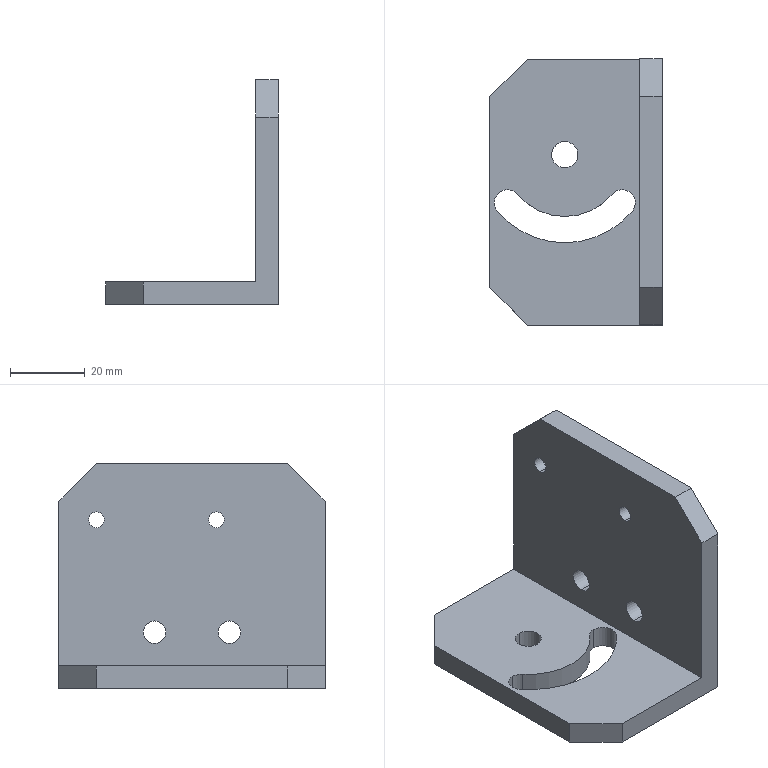Part | SolidWorks | features HoleWzd 3, ICE 2, Chamfer 1, Extrusion 1 | 1 solid | 28 faces | box 46 x 71 x 60 mm | volume 38967 mm3 | cylinder 16 | plane 12 | commonest cylinder face diameters 7 x6 4.2 x4 6 x4 33 x1 47 x1
STEP:
#1=CARTESIAN_POINT('',(-4.679,0.6442,-24.));
#2=VERTEX_POINT('',#1);
#3=CARTESIAN_POINT('',(-1.998,-5.106,-24.));
#4=VERTEX_POINT('',#3);
#5=CARTESIAN_POINT('',(-4.679,-2.856,-24.));
#6=DIRECTION('',(0.,0.,-1.));
#7=DIRECTION('',(0.,1.,0.));
#8=AXIS2_PLACEMENT_3D('',#5,#6,#7);
#9=CIRCLE('',#8,3.5);
#10=EDGE_CURVE('',#2,#4,#9,.T.);
#11=ORIENTED_EDGE('',*,*,#10,.F.);
#12=CARTESIAN_POINT('',(-4.679,0.6442,-30.));
#13=VERTEX_POINT('',#12);
#14=CARTESIAN_POINT('',(-4.679,0.6442,30.));
#15=DIRECTION('',(0.,0.,-1.));
#16=VECTOR('',#15,1000.);
#17=LINE('',#14,#16);
#18=EDGE_CURVE('',#2,#13,#17,.T.);
#19=ORIENTED_EDGE('',*,*,#18,.T.);
#20=CARTESIAN_POINT('',(-1.998,-5.106,-30.));
#21=VERTEX_POINT('',#20);
#22=CARTESIAN_POINT('',(-4.679,-2.856,-30.));
#23=DIRECTION('',(0.,0.,-1.));
#24=DIRECTION('',(0.,1.,0.));
#25=AXIS2_PLACEMENT_3D('',#22,#23,#24);
#26=CIRCLE('',#25,3.5);
#27=EDGE_CURVE('',#13,#21,#26,.T.);
#28=ORIENTED_EDGE('',*,*,#27,.T.);
#29=CARTESIAN_POINT('',(-1.998,-5.106,30.));
#30=DIRECTION('',(0.,0.,-1.));
#31=VECTOR('',#30,1000.);
#32=LINE('',#29,#31);
#33=EDGE_CURVE('',#4,#21,#32,.T.);
#34=ORIENTED_EDGE('',*,*,#33,.F.);
#35=EDGE_LOOP('',(#11,#19,#28,#34));
#36=FACE_OUTER_BOUND('',#35,.T.);
#37=CARTESIAN_POINT('',(-4.679,-2.856,30.));
#38=DIRECTION('',(0.,0.,-1.));
#39=DIRECTION('',(0.,1.,0.));
#40=AXIS2_PLACEMENT_3D('',#37,#38,#39);
#41=CYLINDRICAL_SURFACE('',#40,3.5);
#42=ADVANCED_FACE('',(#36),#41,.F.);
#43=CARTESIAN_POINT('',(-35.321,0.6442,-24.));
#44=VERTEX_POINT('',#43);
#45=CARTESIAN_POINT('',(-32.64,-0.606,-24.));
#46=VERTEX_POINT('',#45);
#47=CARTESIAN_POINT('',(-35.321,-2.856,-24.));
#48=DIRECTION('',(0.,0.,-1.));
#49=DIRECTION('',(0.,1.,0.));
#50=AXIS2_PLACEMENT_3D('',#47,#48,#49);
#51=CIRCLE('',#50,3.5);
#52=EDGE_CURVE('',#44,#46,#51,.T.);
#53=ORIENTED_EDGE('',*,*,#52,.F.);
#54=CARTESIAN_POINT('',(-35.321,0.6442,-30.));
#55=VERTEX_POINT('',#54);
#56=CARTESIAN_POINT('',(-35.321,0.6442,30.));
#57=DIRECTION('',(0.,0.,-1.));
#58=VECTOR('',#57,1000.);
#59=LINE('',#56,#58);
#60=EDGE_CURVE('',#44,#55,#59,.T.);
#61=ORIENTED_EDGE('',*,*,#60,.T.);
#62=CARTESIAN_POINT('',(-32.64,-0.606,-30.));
#63=VERTEX_POINT('',#62);
#64=CARTESIAN_POINT('',(-35.321,-2.856,-30.));
#65=DIRECTION('',(0.,0.,-1.));
#66=DIRECTION('',(0.,1.,0.));
#67=AXIS2_PLACEMENT_3D('',#64,#65,#66);
#68=CIRCLE('',#67,3.5);
#69=EDGE_CURVE('',#55,#63,#68,.T.);
#70=ORIENTED_EDGE('',*,*,#69,.T.);
#71=CARTESIAN_POINT('',(-32.64,-0.606,30.));
#72=DIRECTION('',(0.,0.,-1.));
#73=VECTOR('',#72,1000.);
#74=LINE('',#71,#73);
#75=EDGE_CURVE('',#46,#63,#74,.T.);
#76=ORIENTED_EDGE('',*,*,#75,.F.);
#77=EDGE_LOOP('',(#53,#61,#70,#76));
#78=FACE_OUTER_BOUND('',#77,.T.);
#79=CARTESIAN_POINT('',(-35.321,-2.856,30.));
#80=DIRECTION('',(0.,0.,-1.));
#81=DIRECTION('',(0.,1.,0.));
#82=AXIS2_PLACEMENT_3D('',#79,#80,#81);
#83=CYLINDRICAL_SURFACE('',#82,3.5);
#84=ADVANCED_FACE('',(#78),#83,.F.);
#85=CARTESIAN_POINT('',(-20.,6.5,-24.));
#86=VERTEX_POINT('',#85);
#87=CARTESIAN_POINT('',(-20.,13.5,-24.));
#88=VERTEX_POINT('',#87);
#89=CARTESIAN_POINT('',(-20.,10.,-24.));
#90=DIRECTION('',(0.,0.,-1.));
#91=DIRECTION('',(0.,1.,0.));
#92=AXIS2_PLACEMENT_3D('',#89,#90,#91);
#93=CIRCLE('',#92,3.5);
#94=EDGE_CURVE('',#86,#88,#93,.T.);
#95=ORIENTED_EDGE('',*,*,#94,.F.);
#96=CARTESIAN_POINT('',(-20.,6.5,-30.));
#97=VERTEX_POINT('',#96);
#98=CARTESIAN_POINT('',(-20.,6.5,-30.));
#99=DIRECTION('',(0.,0.,-1.));
#100=VECTOR('',#99,1000.);
#101=LINE('',#98,#100);
#102=EDGE_CURVE('',#86,#97,#101,.T.);
#103=ORIENTED_EDGE('',*,*,#102,.T.);
#104=CARTESIAN_POINT('',(-20.,13.5,-30.));
#105=VERTEX_POINT('',#104);
#106=CARTESIAN_POINT('',(-20.,10.,-30.));
#107=DIRECTION('',(0.,0.,-1.));
#108=DIRECTION('',(0.,1.,0.));
#109=AXIS2_PLACEMENT_3D('',#106,#107,#108);
#110=CIRCLE('',#109,3.5);
#111=EDGE_CURVE('',#97,#105,#110,.T.);
#112=ORIENTED_EDGE('',*,*,#111,.T.);
#113=CARTESIAN_POINT('',(-20.,13.5,-30.));
#114=DIRECTION('',(0.,0.,-1.));
#115=VECTOR('',#114,1000.);
#116=LINE('',#113,#115);
#117=EDGE_CURVE('',#88,#105,#116,.T.);
#118=ORIENTED_EDGE('',*,*,#117,.F.);
#119=EDGE_LOOP('',(#95,#103,#112,#118));
#120=FACE_OUTER_BOUND('',#119,.T.);
#121=CARTESIAN_POINT('',(-20.,10.,-30.));
#122=DIRECTION('',(0.,0.,-1.));
#123=DIRECTION('',(0.,1.,0.));
#124=AXIS2_PLACEMENT_3D('',#121,#122,#123);
#125=CYLINDRICAL_SURFACE('',#124,3.5);
#126=ADVANCED_FACE('',(#120),#125,.F.);
#127=CARTESIAN_POINT('',(6.,10.,-18.));
#128=VERTEX_POINT('',#127);
#129=CARTESIAN_POINT('',(6.,10.,-12.));
#130=VERTEX_POINT('',#129);
#131=CARTESIAN_POINT('',(6.,10.,-15.));
#132=DIRECTION('',(-1.,0.,0.));
#133=DIRECTION('',(0.,0.,1.));
#134=AXIS2_PLACEMENT_3D('',#131,#132,#133);
#135=CIRCLE('',#134,3.);
#136=EDGE_CURVE('',#128,#130,#135,.T.);
#137=ORIENTED_EDGE('',*,*,#136,.F.);
#138=CARTESIAN_POINT('',(0.,10.,-18.));
#139=VERTEX_POINT('',#138);
#140=CARTESIAN_POINT('',(0.,10.,-18.));
#141=DIRECTION('',(-1.,0.,0.));
#142=VECTOR('',#141,1000.);
#143=LINE('',#140,#142);
#144=EDGE_CURVE('',#128,#139,#143,.T.);
#145=ORIENTED_EDGE('',*,*,#144,.T.);
#146=CARTESIAN_POINT('',(0.,10.,-12.));
#147=VERTEX_POINT('',#146);
#148=CARTESIAN_POINT('',(0.,10.,-15.));
#149=DIRECTION('',(-1.,0.,0.));
#150=DIRECTION('',(0.,0.,1.));
#151=AXIS2_PLACEMENT_3D('',#148,#149,#150);
#152=CIRCLE('',#151,3.);
#153=EDGE_CURVE('',#139,#147,#152,.T.);
#154=ORIENTED_EDGE('',*,*,#153,.T.);
#155=CARTESIAN_POINT('',(0.,10.,-12.));
#156=DIRECTION('',(-1.,0.,0.));
#157=VECTOR('',#156,1000.);
#158=LINE('',#155,#157);
#159=EDGE_CURVE('',#130,#147,#158,.T.);
#160=ORIENTED_EDGE('',*,*,#159,.F.);
#161=EDGE_LOOP('',(#137,#145,#154,#160));
#162=FACE_OUTER_BOUND('',#161,.T.);
#163=CARTESIAN_POINT('',(0.,10.,-15.));
#164=DIRECTION('',(-1.,0.,0.));
#165=DIRECTION('',(0.,0.,1.));
#166=AXIS2_PLACEMENT_3D('',#163,#164,#165);
#167=CYLINDRICAL_SURFACE('',#166,3.);
#168=ADVANCED_FACE('',(#162),#167,.F.);
#169=CARTESIAN_POINT('',(6.,-10.,-18.));
#170=VERTEX_POINT('',#169);
#171=CARTESIAN_POINT('',(6.,-10.,-12.));
#172=VERTEX_POINT('',#171);
#173=CARTESIAN_POINT('',(6.,-10.,-15.));
#174=DIRECTION('',(-1.,0.,0.));
#175=DIRECTION('',(0.,0.,1.));
#176=AXIS2_PLACEMENT_3D('',#173,#174,#175);
#177=CIRCLE('',#176,3.);
#178=EDGE_CURVE('',#170,#172,#177,.T.);
#179=ORIENTED_EDGE('',*,*,#178,.F.);
#180=CARTESIAN_POINT('',(0.,-10.,-18.));
#181=VERTEX_POINT('',#180);
#182=CARTESIAN_POINT('',(0.,-10.,-18.));
#183=DIRECTION('',(-1.,0.,0.));
#184=VECTOR('',#183,1000.);
#185=LINE('',#182,#184);
#186=EDGE_CURVE('',#170,#181,#185,.T.);
#187=ORIENTED_EDGE('',*,*,#186,.T.);
#188=CARTESIAN_POINT('',(0.,-10.,-12.));
#189=VERTEX_POINT('',#188);
#190=CARTESIAN_POINT('',(0.,-10.,-15.));
#191=DIRECTION('',(-1.,0.,0.));
#192=DIRECTION('',(0.,0.,1.));
#193=AXIS2_PLACEMENT_3D('',#190,#191,#192);
#194=CIRCLE('',#193,3.);
#195=EDGE_CURVE('',#181,#189,#194,.T.);
#196=ORIENTED_EDGE('',*,*,#195,.T.);
#197=CARTESIAN_POINT('',(0.,-10.,-12.));
#198=DIRECTION('',(-1.,0.,0.));
#199=VECTOR('',#198,1000.);
#200=LINE('',#197,#199);
#201=EDGE_CURVE('',#172,#189,#200,.T.);
#202=ORIENTED_EDGE('',*,*,#201,.F.);
#203=EDGE_LOOP('',(#179,#187,#196,#202));
#204=FACE_OUTER_BOUND('',#203,.T.);
#205=CARTESIAN_POINT('',(0.,-10.,-15.));
#206=DIRECTION('',(-1.,0.,0.));
#207=DIRECTION('',(0.,0.,1.));
#208=AXIS2_PLACEMENT_3D('',#205,#206,#207);
#209=CYLINDRICAL_SURFACE('',#208,3.);
#210=ADVANCED_FACE('',(#204),#209,.F.);
#211=CARTESIAN_POINT('',(0.,25.5,17.1));
#212=VERTEX_POINT('',#211);
#213=CARTESIAN_POINT('',(0.,25.5,12.9));
#214=VERTEX_POINT('',#213);
#215=CARTESIAN_POINT('',(0.,25.5,15.));
#216=DIRECTION('',(1.,0.,0.));
#217=DIRECTION('',(0.,0.,-1.));
#218=AXIS2_PLACEMENT_3D('',#215,#216,#217);
#219=CIRCLE('',#218,2.1);
#220=EDGE_CURVE('',#212,#214,#219,.T.);
#221=ORIENTED_EDGE('',*,*,#220,.F.);
#222=CARTESIAN_POINT('',(6.,25.5,17.1));
#223=VERTEX_POINT('',#222);
#224=CARTESIAN_POINT('',(6.,25.5,17.1));
#225=DIRECTION('',(1.,0.,0.));
#226=VECTOR('',#225,1000.);
#227=LINE('',#224,#226);
#228=EDGE_CURVE('',#212,#223,#227,.T.);
#229=ORIENTED_EDGE('',*,*,#228,.T.);
#230=CARTESIAN_POINT('',(6.,25.5,12.9));
#231=VERTEX_POINT('',#230);
#232=CARTESIAN_POINT('',(6.,25.5,15.));
#233=DIRECTION('',(1.,0.,0.));
#234=DIRECTION('',(0.,0.,-1.));
#235=AXIS2_PLACEMENT_3D('',#232,#233,#234);
#236=CIRCLE('',#235,2.1);
#237=EDGE_CURVE('',#223,#231,#236,.T.);
#238=ORIENTED_EDGE('',*,*,#237,.T.);
#239=CARTESIAN_POINT('',(6.,25.5,12.9));
#240=DIRECTION('',(1.,0.,0.));
#241=VECTOR('',#240,1000.);
#242=LINE('',#239,#241);
#243=EDGE_CURVE('',#214,#231,#242,.T.);
#244=ORIENTED_EDGE('',*,*,#243,.F.);
#245=EDGE_LOOP('',(#221,#229,#238,#244));
#246=FACE_OUTER_BOUND('',#245,.T.);
#247=CARTESIAN_POINT('',(6.,25.5,15.));
#248=DIRECTION('',(1.,0.,0.));
#249=DIRECTION('',(0.,0.,-1.));
#250=AXIS2_PLACEMENT_3D('',#247,#248,#249);
#251=CYLINDRICAL_SURFACE('',#250,2.1);
#252=ADVANCED_FACE('',(#246),#251,.F.);
#253=CARTESIAN_POINT('',(0.,-6.5,17.1));
#254=VERTEX_POINT('',#253);
#255=CARTESIAN_POINT('',(0.,-6.5,12.9));
#256=VERTEX_POINT('',#255);
#257=CARTESIAN_POINT('',(0.,-6.5,15.));
#258=DIRECTION('',(1.,0.,0.));
#259=DIRECTION('',(0.,0.,-1.));
#260=AXIS2_PLACEMENT_3D('',#257,#258,#259);
#261=CIRCLE('',#260,2.1);
#262=EDGE_CURVE('',#254,#256,#261,.T.);
#263=ORIENTED_EDGE('',*,*,#262,.F.);
#264=CARTESIAN_POINT('',(6.,-6.5,17.1));
#265=VERTEX_POINT('',#264);
#266=CARTESIAN_POINT('',(6.,-6.5,17.1));
#267=DIRECTION('',(1.,0.,0.));
#268=VECTOR('',#267,1000.);
#269=LINE('',#266,#268);
#270=EDGE_CURVE('',#254,#265,#269,.T.);
#271=ORIENTED_EDGE('',*,*,#270,.T.);
#272=CARTESIAN_POINT('',(6.,-6.5,12.9));
#273=VERTEX_POINT('',#272);
#274=CARTESIAN_POINT('',(6.,-6.5,15.));
#275=DIRECTION('',(1.,0.,0.));
#276=DIRECTION('',(0.,0.,-1.));
#277=AXIS2_PLACEMENT_3D('',#274,#275,#276);
#278=CIRCLE('',#277,2.1);
#279=EDGE_CURVE('',#265,#273,#278,.T.);
#280=ORIENTED_EDGE('',*,*,#279,.T.);
#281=CARTESIAN_POINT('',(6.,-6.5,12.9));
#282=DIRECTION('',(1.,0.,0.));
#283=VECTOR('',#282,1000.);
#284=LINE('',#281,#283);
#285=EDGE_CURVE('',#256,#273,#284,.T.);
#286=ORIENTED_EDGE('',*,*,#285,.F.);
#287=EDGE_LOOP('',(#263,#271,#280,#286));
#288=FACE_OUTER_BOUND('',#287,.T.);
#289=CARTESIAN_POINT('',(6.,-6.5,15.));
#290=DIRECTION('',(1.,0.,0.));
#291=DIRECTION('',(0.,0.,-1.));
#292=AXIS2_PLACEMENT_3D('',#289,#290,#291);
#293=CYLINDRICAL_SURFACE('',#292,2.1);
#294=ADVANCED_FACE('',(#288),#293,.F.);
#295=CARTESIAN_POINT('',(-20.,10.,-30.));
#296=DIRECTION('',(0.,0.,-1.));
#297=DIRECTION('',(0.,1.,0.));
#298=AXIS2_PLACEMENT_3D('',#295,#296,#297);
#299=CIRCLE('',#298,3.5);
#300=EDGE_CURVE('',#105,#97,#299,.T.);
#301=ORIENTED_EDGE('',*,*,#300,.F.);
#302=ORIENTED_EDGE('',*,*,#111,.F.);
#303=EDGE_LOOP('',(#301,#302));
#304=FACE_BOUND('',#303,.T.);
#305=CARTESIAN_POINT('',(6.,-35.5,-30.));
#306=VERTEX_POINT('',#305);
#307=CARTESIAN_POINT('',(-30.,-35.5,-30.));
#308=VERTEX_POINT('',#307);
#309=CARTESIAN_POINT('',(6.,-35.5,-30.));
#310=DIRECTION('',(-1.,0.,0.));
#311=VECTOR('',#310,1000.);
#312=LINE('',#309,#311);
#313=EDGE_CURVE('',#306,#308,#312,.T.);
#314=ORIENTED_EDGE('',*,*,#313,.T.);
#315=CARTESIAN_POINT('',(-40.,-25.5,-30.));
#316=VERTEX_POINT('',#315);
#317=CARTESIAN_POINT('',(-40.,-25.5,-30.));
#318=DIRECTION('',(-0.7071,0.7071,0.));
#319=VECTOR('',#318,1000.);
#320=LINE('',#317,#319);
#321=EDGE_CURVE('',#308,#316,#320,.T.);
#322=ORIENTED_EDGE('',*,*,#321,.T.);
#323=CARTESIAN_POINT('',(-40.,25.5,-30.));
#324=VERTEX_POINT('',#323);
#325=CARTESIAN_POINT('',(-40.,35.5,-30.));
#326=DIRECTION('',(0.,-1.,0.));
#327=VECTOR('',#326,1000.);
#328=LINE('',#325,#327);
#329=EDGE_CURVE('',#324,#316,#328,.T.);
#330=ORIENTED_EDGE('',*,*,#329,.F.);
#331=CARTESIAN_POINT('',(-30.,35.5,-30.));
#332=VERTEX_POINT('',#331);
#333=CARTESIAN_POINT('',(-40.,25.5,-30.));
#334=DIRECTION('',(0.7071,0.7071,0.));
#335=VECTOR('',#334,1000.);
#336=LINE('',#333,#335);
#337=EDGE_CURVE('',#324,#332,#336,.T.);
#338=ORIENTED_EDGE('',*,*,#337,.T.);
#339=CARTESIAN_POINT('',(6.,35.5,-30.));
#340=VERTEX_POINT('',#339);
#341=CARTESIAN_POINT('',(6.,35.5,-30.));
#342=DIRECTION('',(-1.,0.,0.));
#343=VECTOR('',#342,1000.);
#344=LINE('',#341,#343);
#345=EDGE_CURVE('',#340,#332,#344,.T.);
#346=ORIENTED_EDGE('',*,*,#345,.F.);
#347=CARTESIAN_POINT('',(6.,35.5,-30.));
#348=DIRECTION('',(0.,1.,0.));
#349=VECTOR('',#348,1000.);
#350=LINE('',#347,#349);
#351=EDGE_CURVE('',#306,#340,#350,.T.);
#352=ORIENTED_EDGE('',*,*,#351,.F.);
#353=EDGE_LOOP('',(#314,#322,#330,#338,#346,#352));
#354=FACE_OUTER_BOUND('',#353,.T.);
#355=CARTESIAN_POINT('',(-7.36,-0.606,-30.));
#356=VERTEX_POINT('',#355);
#357=CARTESIAN_POINT('',(-20.,10.,-30.));
#358=DIRECTION('',(0.,0.,1.));
#359=DIRECTION('',(0.,1.,0.));
#360=AXIS2_PLACEMENT_3D('',#357,#358,#359);
#361=CIRCLE('',#360,16.5);
#362=EDGE_CURVE('',#63,#356,#361,.T.);
#363=ORIENTED_EDGE('',*,*,#362,.F.);
#364=ORIENTED_EDGE('',*,*,#69,.F.);
#365=CARTESIAN_POINT('',(-38.002,-5.106,-30.));
#366=VERTEX_POINT('',#365);
#367=CARTESIAN_POINT('',(-35.321,-2.856,-30.));
#368=DIRECTION('',(0.,0.,-1.));
#369=DIRECTION('',(0.,1.,0.));
#370=AXIS2_PLACEMENT_3D('',#367,#368,#369);
#371=CIRCLE('',#370,3.5);
#372=EDGE_CURVE('',#366,#55,#371,.T.);
#373=ORIENTED_EDGE('',*,*,#372,.F.);
#374=CARTESIAN_POINT('',(-20.,10.,-30.));
#375=DIRECTION('',(0.,0.,-1.));
#376=DIRECTION('',(0.,1.,0.));
#377=AXIS2_PLACEMENT_3D('',#374,#375,#376);
#378=CIRCLE('',#377,23.5);
#379=EDGE_CURVE('',#21,#366,#378,.T.);
#380=ORIENTED_EDGE('',*,*,#379,.F.);
#381=ORIENTED_EDGE('',*,*,#27,.F.);
#382=CARTESIAN_POINT('',(-4.679,-2.856,-30.));
#383=DIRECTION('',(0.,0.,-1.));
#384=DIRECTION('',(0.,1.,0.));
#385=AXIS2_PLACEMENT_3D('',#382,#383,#384);
#386=CIRCLE('',#385,3.5);
#387=EDGE_CURVE('',#356,#13,#386,.T.);
#388=ORIENTED_EDGE('',*,*,#387,.F.);
#389=EDGE_LOOP('',(#363,#364,#373,#380,#381,#388));
#390=FACE_BOUND('',#389,.T.);
#391=CARTESIAN_POINT('',(6.,35.5,-30.));
#392=DIRECTION('',(0.,0.,1.));
#393=DIRECTION('',(0.,-1.,0.));
#394=AXIS2_PLACEMENT_3D('',#391,#392,#393);
#395=PLANE('',#394);
#396=ADVANCED_FACE('',(#304,#354,#390),#395,.F.);
#397=CARTESIAN_POINT('',(-20.,10.,-24.));
#398=DIRECTION('',(0.,0.,-1.));
#399=DIRECTION('',(0.,1.,0.));
#400=AXIS2_PLACEMENT_3D('',#397,#398,#399);
#401=CIRCLE('',#400,3.5);
#402=EDGE_CURVE('',#88,#86,#401,.T.);
#403=ORIENTED_EDGE('',*,*,#402,.T.);
#404=ORIENTED_EDGE('',*,*,#94,.T.);
#405=EDGE_LOOP('',(#403,#404));
#406=FACE_BOUND('',#405,.T.);
#407=CARTESIAN_POINT('',(-40.,-25.5,-24.));
#408=VERTEX_POINT('',#407);
#409=CARTESIAN_POINT('',(-40.,25.5,-24.));
#410=VERTEX_POINT('',#409);
#411=CARTESIAN_POINT('',(-40.,35.5,-24.));
#412=DIRECTION('',(0.,1.,0.));
#413=VECTOR('',#412,1000.);
#414=LINE('',#411,#413);
#415=EDGE_CURVE('',#408,#410,#414,.T.);
#416=ORIENTED_EDGE('',*,*,#415,.F.);
#417=CARTESIAN_POINT('',(-30.,-35.5,-24.));
#418=VERTEX_POINT('',#417);
#419=CARTESIAN_POINT('',(-40.,-25.5,-24.));
#420=DIRECTION('',(0.7071,-0.7071,0.));
#421=VECTOR('',#420,1000.);
#422=LINE('',#419,#421);
#423=EDGE_CURVE('',#408,#418,#422,.T.);
#424=ORIENTED_EDGE('',*,*,#423,.T.);
#425=CARTESIAN_POINT('',(0.,-35.5,-24.));
#426=VERTEX_POINT('',#425);
#427=CARTESIAN_POINT('',(-40.,-35.5,-24.));
#428=DIRECTION('',(1.,0.,0.));
#429=VECTOR('',#428,1000.);
#430=LINE('',#427,#429);
#431=EDGE_CURVE('',#418,#426,#430,.T.);
#432=ORIENTED_EDGE('',*,*,#431,.T.);
#433=CARTESIAN_POINT('',(0.,35.5,-24.));
#434=VERTEX_POINT('',#433);
#435=CARTESIAN_POINT('',(0.,35.5,-24.));
#436=DIRECTION('',(0.,1.,0.));
#437=VECTOR('',#436,1000.);
#438=LINE('',#435,#437);
#439=EDGE_CURVE('',#426,#434,#438,.T.);
#440=ORIENTED_EDGE('',*,*,#439,.T.);
#441=CARTESIAN_POINT('',(-30.,35.5,-24.));
#442=VERTEX_POINT('',#441);
#443=CARTESIAN_POINT('',(-40.,35.5,-24.));
#444=DIRECTION('',(1.,0.,0.));
#445=VECTOR('',#444,1000.);
#446=LINE('',#443,#445);
#447=EDGE_CURVE('',#442,#434,#446,.T.);
#448=ORIENTED_EDGE('',*,*,#447,.F.);
#449=CARTESIAN_POINT('',(-40.,25.5,-24.));
#450=DIRECTION('',(-0.7071,-0.7071,0.));
#451=VECTOR('',#450,1000.);
#452=LINE('',#449,#451);
#453=EDGE_CURVE('',#442,#410,#452,.T.);
#454=ORIENTED_EDGE('',*,*,#453,.T.);
#455=EDGE_LOOP('',(#416,#424,#432,#440,#448,#454));
#456=FACE_OUTER_BOUND('',#455,.T.);
#457=CARTESIAN_POINT('',(-38.002,-5.106,-24.));
#458=VERTEX_POINT('',#457);
#459=CARTESIAN_POINT('',(-20.,10.,-24.));
#460=DIRECTION('',(0.,0.,-1.));
#461=DIRECTION('',(0.,1.,0.));
#462=AXIS2_PLACEMENT_3D('',#459,#460,#461);
#463=CIRCLE('',#462,23.5);
#464=EDGE_CURVE('',#4,#458,#463,.T.);
#465=ORIENTED_EDGE('',*,*,#464,.T.);
#466=CARTESIAN_POINT('',(-35.321,-2.856,-24.));
#467=DIRECTION('',(0.,0.,-1.));
#468=DIRECTION('',(0.,1.,0.));
#469=AXIS2_PLACEMENT_3D('',#466,#467,#468);
#470=CIRCLE('',#469,3.5);
#471=EDGE_CURVE('',#458,#44,#470,.T.);
#472=ORIENTED_EDGE('',*,*,#471,.T.);
#473=ORIENTED_EDGE('',*,*,#52,.T.);
#474=CARTESIAN_POINT('',(-7.36,-0.606,-24.));
#475=VERTEX_POINT('',#474);
#476=CARTESIAN_POINT('',(-20.,10.,-24.));
#477=DIRECTION('',(0.,0.,1.));
#478=DIRECTION('',(0.,1.,0.));
#479=AXIS2_PLACEMENT_3D('',#476,#477,#478);
#480=CIRCLE('',#479,16.5);
#481=EDGE_CURVE('',#46,#475,#480,.T.);
#482=ORIENTED_EDGE('',*,*,#481,.T.);
#483=CARTESIAN_POINT('',(-4.679,-2.856,-24.));
#484=DIRECTION('',(0.,0.,-1.));
#485=DIRECTION('',(0.,1.,0.));
#486=AXIS2_PLACEMENT_3D('',#483,#484,#485);
#487=CIRCLE('',#486,3.5);
#488=EDGE_CURVE('',#475,#2,#487,.T.);
#489=ORIENTED_EDGE('',*,*,#488,.T.);
#490=ORIENTED_EDGE('',*,*,#10,.T.);
#491=EDGE_LOOP('',(#465,#472,#473,#482,#489,#490));
#492=FACE_BOUND('',#491,.T.);
#493=CARTESIAN_POINT('',(-40.,35.5,-24.));
#494=DIRECTION('',(0.,0.,-1.));
#495=DIRECTION('',(0.,1.,0.));
#496=AXIS2_PLACEMENT_3D('',#493,#494,#495);
#497=PLANE('',#496);
#498=ADVANCED_FACE('',(#406,#456,#492),#497,.F.);
#499=CARTESIAN_POINT('',(0.,-6.5,15.));
#500=DIRECTION('',(1.,0.,0.));
#501=DIRECTION('',(0.,0.,-1.));
#502=AXIS2_PLACEMENT_3D('',#499,#500,#501);
#503=CIRCLE('',#502,2.1);
#504=EDGE_CURVE('',#256,#254,#503,.T.);
#505=ORIENTED_EDGE('',*,*,#504,.T.);
#506=ORIENTED_EDGE('',*,*,#262,.T.);
#507=EDGE_LOOP('',(#505,#506));
#508=FACE_BOUND('',#507,.T.);
#509=CARTESIAN_POINT('',(0.,25.5,15.));
#510=DIRECTION('',(1.,0.,0.));
#511=DIRECTION('',(0.,0.,-1.));
#512=AXIS2_PLACEMENT_3D('',#509,#510,#511);
#513=CIRCLE('',#512,2.1);
#514=EDGE_CURVE('',#214,#212,#513,.T.);
#515=ORIENTED_EDGE('',*,*,#514,.T.);
#516=ORIENTED_EDGE('',*,*,#220,.T.);
#517=EDGE_LOOP('',(#515,#516));
#518=FACE_BOUND('',#517,.T.);
#519=CARTESIAN_POINT('',(0.,-10.,-15.));
#520=DIRECTION('',(-1.,0.,0.));
#521=DIRECTION('',(0.,0.,1.));
#522=AXIS2_PLACEMENT_3D('',#519,#520,#521);
#523=CIRCLE('',#522,3.);
#524=EDGE_CURVE('',#189,#181,#523,.T.);
#525=ORIENTED_EDGE('',*,*,#524,.F.);
#526=ORIENTED_EDGE('',*,*,#195,.F.);
#527=EDGE_LOOP('',(#525,#526));
#528=FACE_BOUND('',#527,.T.);
#529=CARTESIAN_POINT('',(0.,10.,-15.));
#530=DIRECTION('',(-1.,0.,0.));
#531=DIRECTION('',(0.,0.,1.));
#532=AXIS2_PLACEMENT_3D('',#529,#530,#531);
#533=CIRCLE('',#532,3.);
#534=EDGE_CURVE('',#147,#139,#533,.T.);
#535=ORIENTED_EDGE('',*,*,#534,.F.);
#536=ORIENTED_EDGE('',*,*,#153,.F.);
#537=EDGE_LOOP('',(#535,#536));
#538=FACE_BOUND('',#537,.T.);
#539=CARTESIAN_POINT('',(0.,-35.5,20.));
#540=VERTEX_POINT('',#539);
#541=CARTESIAN_POINT('',(0.,-35.5,30.));
#542=DIRECTION('',(0.,0.,-1.));
#543=VECTOR('',#542,1000.);
#544=LINE('',#541,#543);
#545=EDGE_CURVE('',#540,#426,#544,.T.);
#546=ORIENTED_EDGE('',*,*,#545,.F.);
#547=CARTESIAN_POINT('',(0.,-25.5,30.));
#548=VERTEX_POINT('',#547);
#549=CARTESIAN_POINT('',(0.,-35.5,20.));
#550=DIRECTION('',(0.,0.7071,0.7071));
#551=VECTOR('',#550,1000.);
#552=LINE('',#549,#551);
#553=EDGE_CURVE('',#540,#548,#552,.T.);
#554=ORIENTED_EDGE('',*,*,#553,.T.);
#555=CARTESIAN_POINT('',(0.,25.5,30.));
#556=VERTEX_POINT('',#555);
#557=CARTESIAN_POINT('',(0.,35.5,30.));
#558=DIRECTION('',(0.,-1.,0.));
#559=VECTOR('',#558,1000.);
#560=LINE('',#557,#559);
#561=EDGE_CURVE('',#556,#548,#560,.T.);
#562=ORIENTED_EDGE('',*,*,#561,.F.);
#563=CARTESIAN_POINT('',(0.,35.5,20.));
#564=VERTEX_POINT('',#563);
#565=CARTESIAN_POINT('',(0.,25.5,30.));
#566=DIRECTION('',(0.,0.7071,-0.7071));
#567=VECTOR('',#566,1000.);
#568=LINE('',#565,#567);
#569=EDGE_CURVE('',#556,#564,#568,.T.);
#570=ORIENTED_EDGE('',*,*,#569,.T.);
#571=CARTESIAN_POINT('',(0.,35.5,30.));
#572=DIRECTION('',(0.,0.,1.));
#573=VECTOR('',#572,1000.);
#574=LINE('',#571,#573);
#575=EDGE_CURVE('',#434,#564,#574,.T.);
#576=ORIENTED_EDGE('',*,*,#575,.F.);
#577=ORIENTED_EDGE('',*,*,#439,.F.);
#578=EDGE_LOOP('',(#546,#554,#562,#570,#576,#577));
#579=FACE_OUTER_BOUND('',#578,.T.);
#580=CARTESIAN_POINT('',(0.,0.,0.));
#581=DIRECTION('',(1.,0.,0.));
#582=DIRECTION('',(0.,0.,-1.));
#583=AXIS2_PLACEMENT_3D('',#580,#581,#582);
#584=PLANE('',#583);
#585=ADVANCED_FACE('',(#508,#518,#528,#538,#579),#584,.F.);
#586=ORIENTED_EDGE('',*,*,#575,.T.);
#587=CARTESIAN_POINT('',(6.,35.5,20.));
#588=VERTEX_POINT('',#587);
#589=CARTESIAN_POINT('',(6.,35.5,20.));
#590=DIRECTION('',(1.,0.,0.));
#591=VECTOR('',#590,1000.);
#592=LINE('',#589,#591);
#593=EDGE_CURVE('',#564,#588,#592,.T.);
#594=ORIENTED_EDGE('',*,*,#593,.T.);
#595=CARTESIAN_POINT('',(6.,35.5,30.));
#596=DIRECTION('',(0.,0.,1.));
#597=VECTOR('',#596,1000.);
#598=LINE('',#595,#597);
#599=EDGE_CURVE('',#340,#588,#598,.T.);
#600=ORIENTED_EDGE('',*,*,#599,.F.);
#601=ORIENTED_EDGE('',*,*,#345,.T.);
#602=CARTESIAN_POINT('',(-30.,35.5,-24.));
#603=DIRECTION('',(0.,0.,1.));
#604=VECTOR('',#603,1000.);
#605=LINE('',#602,#604);
#606=EDGE_CURVE('',#332,#442,#605,.T.);
#607=ORIENTED_EDGE('',*,*,#606,.T.);
#608=ORIENTED_EDGE('',*,*,#447,.T.);
#609=EDGE_LOOP('',(#586,#594,#600,#601,#607,#608));
#610=FACE_OUTER_BOUND('',#609,.T.);
#611=CARTESIAN_POINT('',(6.,35.5,30.));
#612=DIRECTION('',(0.,-1.,0.));
#613=DIRECTION('',(0.,0.,-1.));
#614=AXIS2_PLACEMENT_3D('',#611,#612,#613);
#615=PLANE('',#614);
#616=ADVANCED_FACE('',(#610),#615,.F.);
#617=ORIENTED_EDGE('',*,*,#561,.T.);
#618=CARTESIAN_POINT('',(6.,-25.5,30.));
#619=VERTEX_POINT('',#618);
#620=CARTESIAN_POINT('',(6.,-25.5,30.));
#621=DIRECTION('',(1.,0.,0.));
#622=VECTOR('',#621,1000.);
#623=LINE('',#620,#622);
#624=EDGE_CURVE('',#548,#619,#623,.T.);
#625=ORIENTED_EDGE('',*,*,#624,.T.);
#626=CARTESIAN_POINT('',(6.,25.5,30.));
#627=VERTEX_POINT('',#626);
#628=CARTESIAN_POINT('',(6.,35.5,30.));
#629=DIRECTION('',(0.,-1.,0.));
#630=VECTOR('',#629,1000.);
#631=LINE('',#628,#630);
#632=EDGE_CURVE('',#627,#619,#631,.T.);
#633=ORIENTED_EDGE('',*,*,#632,.F.);
#634=CARTESIAN_POINT('',(6.,25.5,30.));
#635=DIRECTION('',(-1.,0.,0.));
#636=VECTOR('',#635,1000.);
#637=LINE('',#634,#636);
#638=EDGE_CURVE('',#627,#556,#637,.T.);
#639=ORIENTED_EDGE('',*,*,#638,.T.);
#640=EDGE_LOOP('',(#617,#625,#633,#639));
#641=FACE_OUTER_BOUND('',#640,.T.);
#642=CARTESIAN_POINT('',(6.,35.5,30.));
#643=DIRECTION('',(0.,0.,-1.));
#644=DIRECTION('',(0.,1.,0.));
#645=AXIS2_PLACEMENT_3D('',#642,#643,#644);
#646=PLANE('',#645);
#647=ADVANCED_FACE('',(#641),#646,.F.);
#648=CARTESIAN_POINT('',(6.,-35.5,20.));
#649=VERTEX_POINT('',#648);
#650=CARTESIAN_POINT('',(6.,-35.5,30.));
#651=DIRECTION('',(0.,0.,-1.));
#652=VECTOR('',#651,1000.);
#653=LINE('',#650,#652);
#654=EDGE_CURVE('',#649,#306,#653,.T.);
#655=ORIENTED_EDGE('',*,*,#654,.F.);
#656=CARTESIAN_POINT('',(6.,-35.5,20.));
#657=DIRECTION('',(-1.,0.,0.));
#658=VECTOR('',#657,1000.);
#659=LINE('',#656,#658);
#660=EDGE_CURVE('',#649,#540,#659,.T.);
#661=ORIENTED_EDGE('',*,*,#660,.T.);
#662=ORIENTED_EDGE('',*,*,#545,.T.);
#663=ORIENTED_EDGE('',*,*,#431,.F.);
#664=CARTESIAN_POINT('',(-30.,-35.5,-30.));
#665=DIRECTION('',(0.,0.,-1.));
#666=VECTOR('',#665,1000.);
#667=LINE('',#664,#666);
#668=EDGE_CURVE('',#418,#308,#667,.T.);
#669=ORIENTED_EDGE('',*,*,#668,.T.);
#670=ORIENTED_EDGE('',*,*,#313,.F.);
#671=EDGE_LOOP('',(#655,#661,#662,#663,#669,#670));
#672=FACE_OUTER_BOUND('',#671,.T.);
#673=CARTESIAN_POINT('',(6.,-35.5,30.));
#674=DIRECTION('',(0.,1.,0.));
#675=DIRECTION('',(0.,0.,1.));
#676=AXIS2_PLACEMENT_3D('',#673,#674,#675);
#677=PLANE('',#676);
#678=ADVANCED_FACE('',(#672),#677,.F.);
#679=CARTESIAN_POINT('',(6.,10.,-15.));
#680=DIRECTION('',(-1.,0.,0.));
#681=DIRECTION('',(0.,0.,1.));
#682=AXIS2_PLACEMENT_3D('',#679,#680,#681);
#683=CIRCLE('',#682,3.);
#684=EDGE_CURVE('',#130,#128,#683,.T.);
#685=ORIENTED_EDGE('',*,*,#684,.T.);
#686=ORIENTED_EDGE('',*,*,#136,.T.);
#687=EDGE_LOOP('',(#685,#686));
#688=FACE_BOUND('',#687,.T.);
#689=CARTESIAN_POINT('',(6.,-10.,-15.));
#690=DIRECTION('',(-1.,0.,0.));
#691=DIRECTION('',(0.,0.,1.));
#692=AXIS2_PLACEMENT_3D('',#689,#690,#691);
#693=CIRCLE('',#692,3.);
#694=EDGE_CURVE('',#172,#170,#693,.T.);
#695=ORIENTED_EDGE('',*,*,#694,.T.);
#696=ORIENTED_EDGE('',*,*,#178,.T.);
#697=EDGE_LOOP('',(#695,#696));
#698=FACE_BOUND('',#697,.T.);
#699=CARTESIAN_POINT('',(6.,25.5,15.));
#700=DIRECTION('',(1.,0.,0.));
#701=DIRECTION('',(0.,0.,-1.));
#702=AXIS2_PLACEMENT_3D('',#699,#700,#701);
#703=CIRCLE('',#702,2.1);
#704=EDGE_CURVE('',#231,#223,#703,.T.);
#705=ORIENTED_EDGE('',*,*,#704,.F.);
#706=ORIENTED_EDGE('',*,*,#237,.F.);
#707=EDGE_LOOP('',(#705,#706));
#708=FACE_BOUND('',#707,.T.);
#709=CARTESIAN_POINT('',(6.,-6.5,15.));
#710=DIRECTION('',(1.,0.,0.));
#711=DIRECTION('',(0.,0.,-1.));
#712=AXIS2_PLACEMENT_3D('',#709,#710,#711);
#713=CIRCLE('',#712,2.1);
#714=EDGE_CURVE('',#273,#265,#713,.T.);
#715=ORIENTED_EDGE('',*,*,#714,.F.);
#716=ORIENTED_EDGE('',*,*,#279,.F.);
#717=EDGE_LOOP('',(#715,#716));
#718=FACE_BOUND('',#717,.T.);
#719=ORIENTED_EDGE('',*,*,#632,.T.);
#720=CARTESIAN_POINT('',(6.,-27.75,27.75));
#721=DIRECTION('',(0.,-0.7071,-0.7071));
#722=VECTOR('',#721,1000.);
#723=LINE('',#720,#722);
#724=EDGE_CURVE('',#619,#649,#723,.T.);
#725=ORIENTED_EDGE('',*,*,#724,.T.);
#726=ORIENTED_EDGE('',*,*,#654,.T.);
#727=ORIENTED_EDGE('',*,*,#351,.T.);
#728=ORIENTED_EDGE('',*,*,#599,.T.);
#729=CARTESIAN_POINT('',(6.,27.75,27.75));
#730=DIRECTION('',(0.,-0.7071,0.7071));
#731=VECTOR('',#730,1000.);
#732=LINE('',#729,#731);
#733=EDGE_CURVE('',#588,#627,#732,.T.);
#734=ORIENTED_EDGE('',*,*,#733,.T.);
#735=EDGE_LOOP('',(#719,#725,#726,#727,#728,#734));
#736=FACE_OUTER_BOUND('',#735,.T.);
#737=CARTESIAN_POINT('',(6.,0.,0.));
#738=DIRECTION('',(1.,0.,0.));
#739=DIRECTION('',(0.,0.,-1.));
#740=AXIS2_PLACEMENT_3D('',#737,#738,#739);
#741=PLANE('',#740);
#742=ADVANCED_FACE('',(#688,#698,#708,#718,#736),#741,.T.);
#743=ORIENTED_EDGE('',*,*,#270,.F.);
#744=ORIENTED_EDGE('',*,*,#504,.F.);
#745=ORIENTED_EDGE('',*,*,#285,.T.);
#746=ORIENTED_EDGE('',*,*,#714,.T.);
#747=EDGE_LOOP('',(#743,#744,#745,#746));
#748=FACE_OUTER_BOUND('',#747,.T.);
#749=CARTESIAN_POINT('',(6.,-6.5,15.));
#750=DIRECTION('',(1.,0.,0.));
#751=DIRECTION('',(0.,0.,-1.));
#752=AXIS2_PLACEMENT_3D('',#749,#750,#751);
#753=CYLINDRICAL_SURFACE('',#752,2.1);
#754=ADVANCED_FACE('',(#748),#753,.F.);
#755=ORIENTED_EDGE('',*,*,#228,.F.);
#756=ORIENTED_EDGE('',*,*,#514,.F.);
#757=ORIENTED_EDGE('',*,*,#243,.T.);
#758=ORIENTED_EDGE('',*,*,#704,.T.);
#759=EDGE_LOOP('',(#755,#756,#757,#758));
#760=FACE_OUTER_BOUND('',#759,.T.);
#761=CARTESIAN_POINT('',(6.,25.5,15.));
#762=DIRECTION('',(1.,0.,0.));
#763=DIRECTION('',(0.,0.,-1.));
#764=AXIS2_PLACEMENT_3D('',#761,#762,#763);
#765=CYLINDRICAL_SURFACE('',#764,2.1);
#766=ADVANCED_FACE('',(#760),#765,.F.);
#767=ORIENTED_EDGE('',*,*,#186,.F.);
#768=ORIENTED_EDGE('',*,*,#694,.F.);
#769=ORIENTED_EDGE('',*,*,#201,.T.);
#770=ORIENTED_EDGE('',*,*,#524,.T.);
#771=EDGE_LOOP('',(#767,#768,#769,#770));
#772=FACE_OUTER_BOUND('',#771,.T.);
#773=CARTESIAN_POINT('',(0.,-10.,-15.));
#774=DIRECTION('',(-1.,0.,0.));
#775=DIRECTION('',(0.,0.,1.));
#776=AXIS2_PLACEMENT_3D('',#773,#774,#775);
#777=CYLINDRICAL_SURFACE('',#776,3.);
#778=ADVANCED_FACE('',(#772),#777,.F.);
#779=ORIENTED_EDGE('',*,*,#144,.F.);
#780=ORIENTED_EDGE('',*,*,#684,.F.);
#781=ORIENTED_EDGE('',*,*,#159,.T.);
#782=ORIENTED_EDGE('',*,*,#534,.T.);
#783=EDGE_LOOP('',(#779,#780,#781,#782));
#784=FACE_OUTER_BOUND('',#783,.T.);
#785=CARTESIAN_POINT('',(0.,10.,-15.));
#786=DIRECTION('',(-1.,0.,0.));
#787=DIRECTION('',(0.,0.,1.));
#788=AXIS2_PLACEMENT_3D('',#785,#786,#787);
#789=CYLINDRICAL_SURFACE('',#788,3.);
#790=ADVANCED_FACE('',(#784),#789,.F.);
#791=ORIENTED_EDGE('',*,*,#329,.T.);
#792=CARTESIAN_POINT('',(-40.,-25.5,-24.));
#793=DIRECTION('',(0.,0.,1.));
#794=VECTOR('',#793,1000.);
#795=LINE('',#792,#794);
#796=EDGE_CURVE('',#316,#408,#795,.T.);
#797=ORIENTED_EDGE('',*,*,#796,.T.);
#798=ORIENTED_EDGE('',*,*,#415,.T.);
#799=CARTESIAN_POINT('',(-40.,25.5,-30.));
#800=DIRECTION('',(0.,0.,-1.));
#801=VECTOR('',#800,1000.);
#802=LINE('',#799,#801);
#803=EDGE_CURVE('',#410,#324,#802,.T.);
#804=ORIENTED_EDGE('',*,*,#803,.T.);
#805=EDGE_LOOP('',(#791,#797,#798,#804));
#806=FACE_OUTER_BOUND('',#805,.T.);
#807=CARTESIAN_POINT('',(-40.,0.,0.));
#808=DIRECTION('',(-1.,0.,0.));
#809=DIRECTION('',(0.,0.,1.));
#810=AXIS2_PLACEMENT_3D('',#807,#808,#809);
#811=PLANE('',#810);
#812=ADVANCED_FACE('',(#806),#811,.T.);
#813=ORIENTED_EDGE('',*,*,#102,.F.);
#814=ORIENTED_EDGE('',*,*,#402,.F.);
#815=ORIENTED_EDGE('',*,*,#117,.T.);
#816=ORIENTED_EDGE('',*,*,#300,.T.);
#817=EDGE_LOOP('',(#813,#814,#815,#816));
#818=FACE_OUTER_BOUND('',#817,.T.);
#819=CARTESIAN_POINT('',(-20.,10.,-30.));
#820=DIRECTION('',(0.,0.,-1.));
#821=DIRECTION('',(0.,1.,0.));
#822=AXIS2_PLACEMENT_3D('',#819,#820,#821);
#823=CYLINDRICAL_SURFACE('',#822,3.5);
#824=ADVANCED_FACE('',(#818),#823,.F.);
#825=ORIENTED_EDGE('',*,*,#60,.F.);
#826=ORIENTED_EDGE('',*,*,#471,.F.);
#827=CARTESIAN_POINT('',(-38.002,-5.106,30.));
#828=DIRECTION('',(0.,0.,-1.));
#829=VECTOR('',#828,1000.);
#830=LINE('',#827,#829);
#831=EDGE_CURVE('',#458,#366,#830,.T.);
#832=ORIENTED_EDGE('',*,*,#831,.T.);
#833=ORIENTED_EDGE('',*,*,#372,.T.);
#834=EDGE_LOOP('',(#825,#826,#832,#833));
#835=FACE_OUTER_BOUND('',#834,.T.);
#836=CARTESIAN_POINT('',(-35.321,-2.856,30.));
#837=DIRECTION('',(0.,0.,-1.));
#838=DIRECTION('',(0.,1.,0.));
#839=AXIS2_PLACEMENT_3D('',#836,#837,#838);
#840=CYLINDRICAL_SURFACE('',#839,3.5);
#841=ADVANCED_FACE('',(#835),#840,.F.);
#842=ORIENTED_EDGE('',*,*,#33,.T.);
#843=ORIENTED_EDGE('',*,*,#379,.T.);
#844=ORIENTED_EDGE('',*,*,#831,.F.);
#845=ORIENTED_EDGE('',*,*,#464,.F.);
#846=EDGE_LOOP('',(#842,#843,#844,#845));
#847=FACE_OUTER_BOUND('',#846,.T.);
#848=CARTESIAN_POINT('',(-20.,10.,30.));
#849=DIRECTION('',(0.,0.,-1.));
#850=DIRECTION('',(0.,1.,0.));
#851=AXIS2_PLACEMENT_3D('',#848,#849,#850);
#852=CYLINDRICAL_SURFACE('',#851,23.5);
#853=ADVANCED_FACE('',(#847),#852,.F.);
#854=ORIENTED_EDGE('',*,*,#18,.F.);
#855=ORIENTED_EDGE('',*,*,#488,.F.);
#856=CARTESIAN_POINT('',(-7.36,-0.606,30.));
#857=DIRECTION('',(0.,0.,-1.));
#858=VECTOR('',#857,1000.);
#859=LINE('',#856,#858);
#860=EDGE_CURVE('',#475,#356,#859,.T.);
#861=ORIENTED_EDGE('',*,*,#860,.T.);
#862=ORIENTED_EDGE('',*,*,#387,.T.);
#863=EDGE_LOOP('',(#854,#855,#861,#862));
#864=FACE_OUTER_BOUND('',#863,.T.);
#865=CARTESIAN_POINT('',(-4.679,-2.856,30.));
#866=DIRECTION('',(0.,0.,-1.));
#867=DIRECTION('',(0.,1.,0.));
#868=AXIS2_PLACEMENT_3D('',#865,#866,#867);
#869=CYLINDRICAL_SURFACE('',#868,3.5);
#870=ADVANCED_FACE('',(#864),#869,.F.);
#871=ORIENTED_EDGE('',*,*,#75,.T.);
#872=ORIENTED_EDGE('',*,*,#362,.T.);
#873=ORIENTED_EDGE('',*,*,#860,.F.);
#874=ORIENTED_EDGE('',*,*,#481,.F.);
#875=EDGE_LOOP('',(#871,#872,#873,#874));
#876=FACE_OUTER_BOUND('',#875,.T.);
#877=CARTESIAN_POINT('',(-20.,10.,30.));
#878=DIRECTION('',(0.,0.,-1.));
#879=DIRECTION('',(0.,1.,0.));
#880=AXIS2_PLACEMENT_3D('',#877,#878,#879);
#881=CYLINDRICAL_SURFACE('',#880,16.5);
#882=ADVANCED_FACE('',(#876),#881,.T.);
#883=ORIENTED_EDGE('',*,*,#724,.F.);
#884=ORIENTED_EDGE('',*,*,#624,.F.);
#885=ORIENTED_EDGE('',*,*,#553,.F.);
#886=ORIENTED_EDGE('',*,*,#660,.F.);
#887=EDGE_LOOP('',(#883,#884,#885,#886));
#888=FACE_OUTER_BOUND('',#887,.T.);
#889=CARTESIAN_POINT('',(6.,-35.5,20.));
#890=DIRECTION('',(0.,0.7071,-0.7071));
#891=DIRECTION('',(-1.,0.,0.));
#892=AXIS2_PLACEMENT_3D('',#889,#890,#891);
#893=PLANE('',#892);
#894=ADVANCED_FACE('',(#888),#893,.F.);
#895=ORIENTED_EDGE('',*,*,#733,.F.);
#896=ORIENTED_EDGE('',*,*,#593,.F.);
#897=ORIENTED_EDGE('',*,*,#569,.F.);
#898=ORIENTED_EDGE('',*,*,#638,.F.);
#899=EDGE_LOOP('',(#895,#896,#897,#898));
#900=FACE_OUTER_BOUND('',#899,.T.);
#901=CARTESIAN_POINT('',(6.,25.5,30.));
#902=DIRECTION('',(0.,-0.7071,-0.7071));
#903=DIRECTION('',(-1.,0.,0.));
#904=AXIS2_PLACEMENT_3D('',#901,#902,#903);
#905=PLANE('',#904);
#906=ADVANCED_FACE('',(#900),#905,.F.);
#907=ORIENTED_EDGE('',*,*,#321,.F.);
#908=ORIENTED_EDGE('',*,*,#668,.F.);
#909=ORIENTED_EDGE('',*,*,#423,.F.);
#910=ORIENTED_EDGE('',*,*,#796,.F.);
#911=EDGE_LOOP('',(#907,#908,#909,#910));
#912=FACE_OUTER_BOUND('',#911,.T.);
#913=CARTESIAN_POINT('',(-40.,-25.5,0.));
#914=DIRECTION('',(-0.7071,-0.7071,0.));
#915=DIRECTION('',(0.,0.,-1.));
#916=AXIS2_PLACEMENT_3D('',#913,#914,#915);
#917=PLANE('',#916);
#918=ADVANCED_FACE('',(#912),#917,.T.);
#919=ORIENTED_EDGE('',*,*,#453,.F.);
#920=ORIENTED_EDGE('',*,*,#606,.F.);
#921=ORIENTED_EDGE('',*,*,#337,.F.);
#922=ORIENTED_EDGE('',*,*,#803,.F.);
#923=EDGE_LOOP('',(#919,#920,#921,#922));
#924=FACE_OUTER_BOUND('',#923,.T.);
#925=CARTESIAN_POINT('',(-40.,25.5,0.));
#926=DIRECTION('',(-0.7071,0.7071,0.));
#927=DIRECTION('',(0.,0.,1.));
#928=AXIS2_PLACEMENT_3D('',#925,#926,#927);
#929=PLANE('',#928);
#930=ADVANCED_FACE('',(#924),#929,.T.);
#931=CLOSED_SHELL('',(#42,#84,#126,#168,#210,#252,#294,#396,#498,#585,#616,#647,#678,#742,#754,#766,#778,#790,#812,#824,#841,#853,#870,#882,#894,#906,#918,#930));
#932=MANIFOLD_SOLID_BREP('',#931);
#933=CARTESIAN_POINT('',(0.,0.,0.));
#934=DIRECTION('',(0.,0.,1.));
#935=DIRECTION('',(1.,0.,0.));
#936=AXIS2_PLACEMENT_3D('',#933,#934,#935);
#937=(LENGTH_UNIT()NAMED_UNIT(*)SI_UNIT(.MILLI.,.METRE.));
#938=UNCERTAINTY_MEASURE_WITH_UNIT(LENGTH_MEASURE(0.00001),#937,'','');
#939=(NAMED_UNIT(*)PLANE_ANGLE_UNIT()SI_UNIT($,.RADIAN.));
#940=(NAMED_UNIT(*)SI_UNIT($,.STERADIAN.)SOLID_ANGLE_UNIT());
#941=(GEOMETRIC_REPRESENTATION_CONTEXT(3)GLOBAL_UNCERTAINTY_ASSIGNED_CONTEXT((#938))GLOBAL_UNIT_ASSIGNED_CONTEXT((#937,#939,#940))REPRESENTATION_CONTEXT('',''));
#942=ADVANCED_BREP_SHAPE_REPRESENTATION('',(#932,#936),#941);